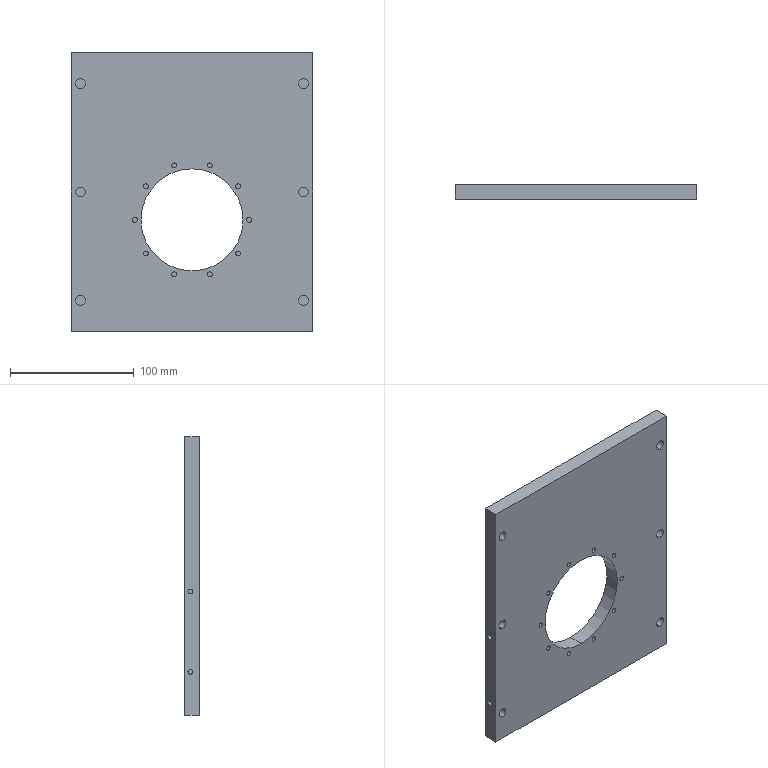Part | STEP file | 2026.6.15-Main Assembly图.sldasm-Part-137 | 1 solid | 62 faces | box 195 x 12 x 225 mm | volume 457954 mm3 | cylinder 38 | plane 24 | commonest cylinder face diameters 4 x24 8 x12 82.5 x2